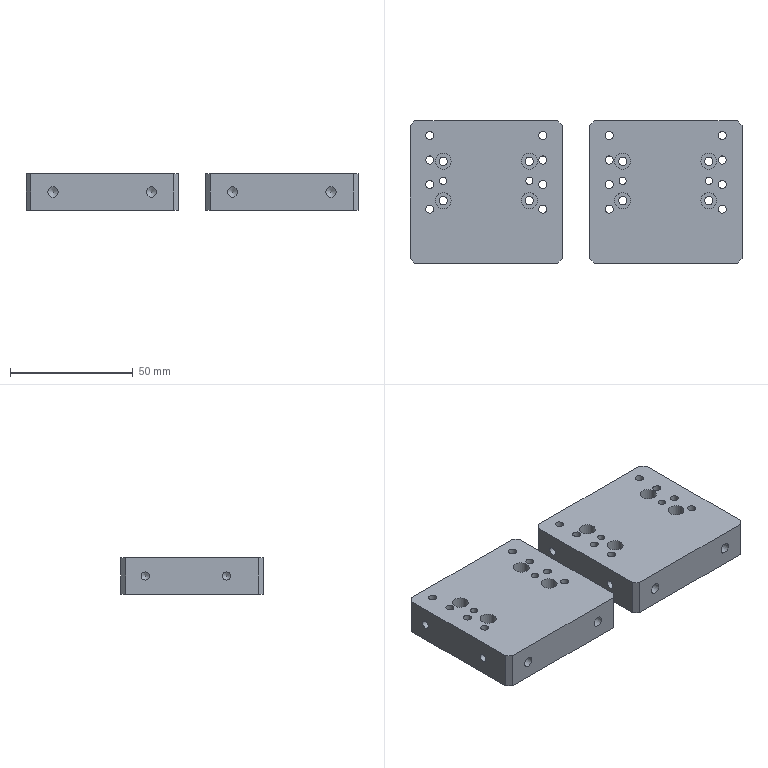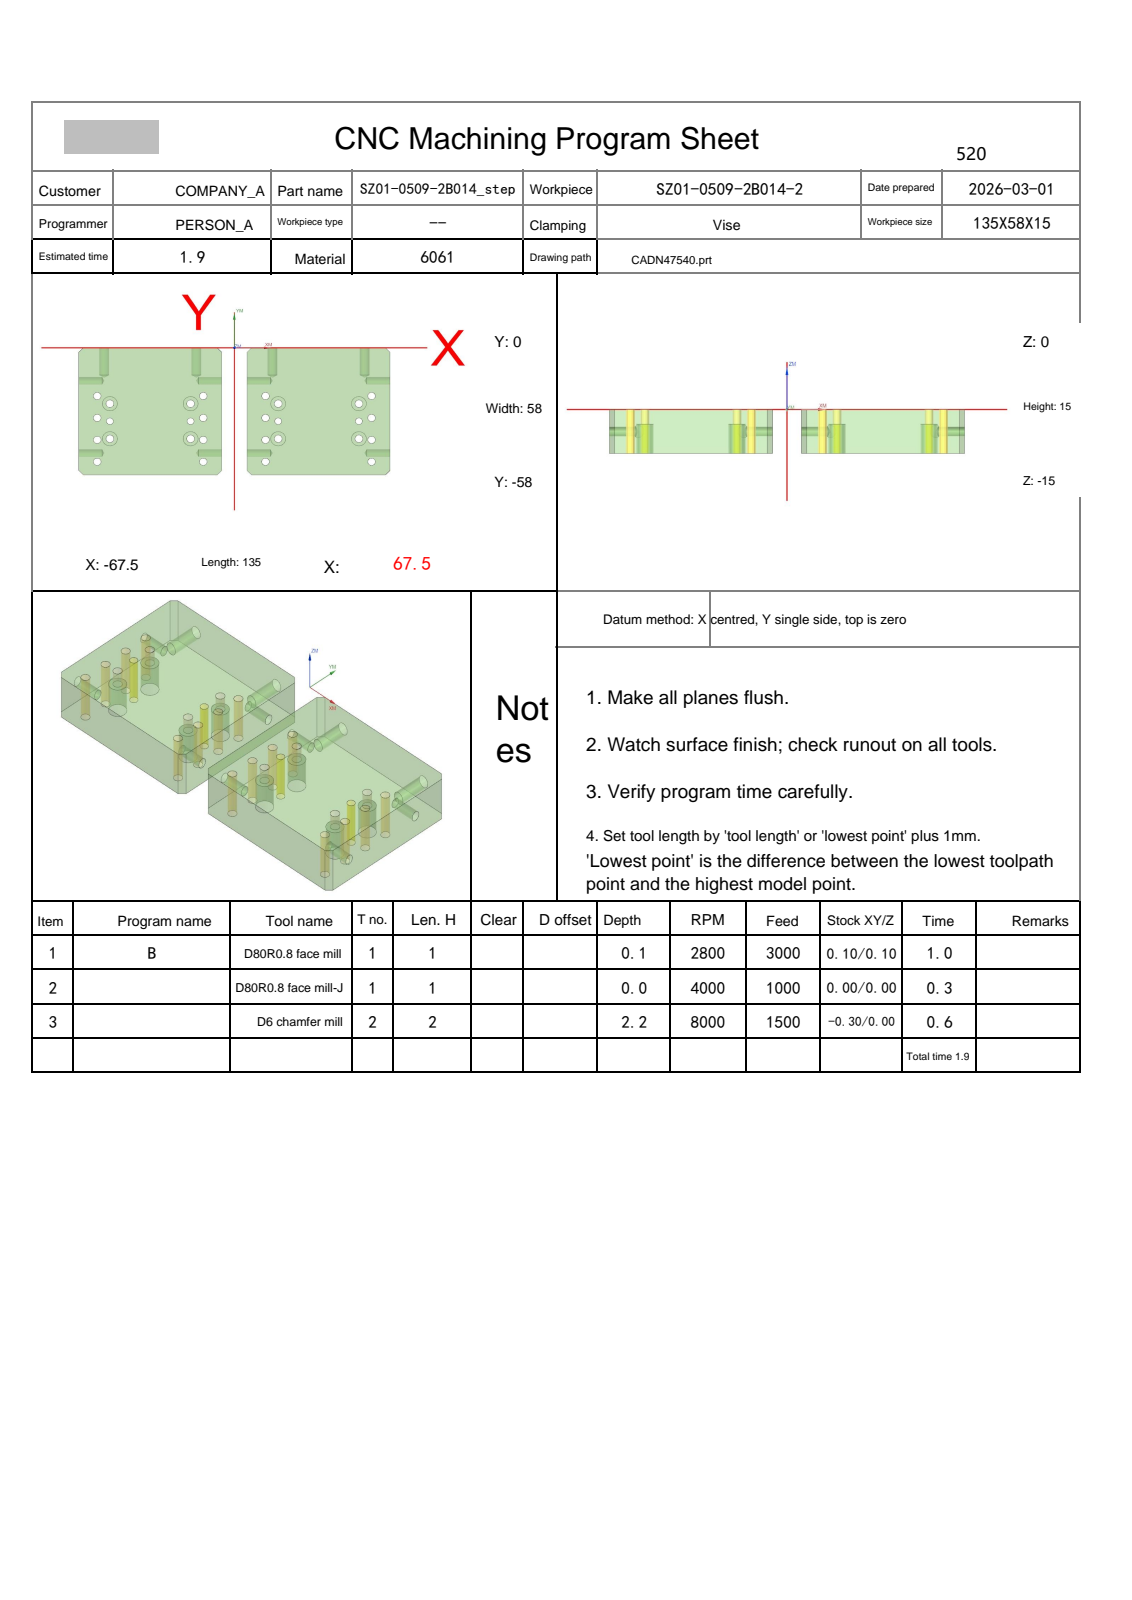NC program | NX | posted by the shop | part box 135 x 58 x 15 mm
Whole program:
%
O0001
(Machine time: 2.35 MIN)
(===Total Tool:2===)
(T1=D80R0.8 face mill D=80.  R=0.8  D-  H01 Z=0.    )
(T2=D6 chamfer mill   D=6.   R=0.   D-  H02 Z=-2.2  )
G80 G90 G17 G49 G40
G91 G28 Z0
M01
N1 T01 M06
(D80R0.8 face mill  D=80. R=0.8 H=01 ce=0.10 di=0.10)
G00 G90 G54 X119.597 Y-29. M03 S2800
G43 H01 Z50.
M08
Z6.011
G01 Z4.011 F3000.
X107.597
X-107.597
X-119.597
Z6.011
G00 X119.597
Z5.522
G01 Z3.522
X107.597
X-107.597
X-119.597
Z5.522
G00 X119.597
Z5.033
G01 Z3.033
X107.597
X-107.597
X-119.597
Z5.033
G00 X119.597
Z4.544
G01 Z2.544
X107.597
X-107.597
X-119.597
Z4.544
G00 Z50.
X119.597
Z4.056
G01 Z2.056
X107.597
X-107.597
X-119.597
Z4.056
G00 Z50.
X119.597
Z3.567
G01 Z1.567
X107.597
X-107.597
X-119.597
Z3.567
G00 Z50.
X119.597
Z3.078
G01 Z1.078
X107.597
X-107.597
X-119.597
Z3.078
G00 Z50.
X119.597
Z2.589
G01 Z.589
X107.597
X-107.597
X-119.597
Z2.589
G00 Z50.
X119.597
Z2.1
G01 Z.1
X107.597
X-107.597
X-119.597
Z2.1
G00 Z50.
G91 G28 Z0.0
M05
M09
G91 G28 Z0.0
M01
N2 T01 M06
(D80R0.8 face mill-J  D=80. R=0.8 H=01 ce=0.00 di=0.00)
G00 G90 G54 X119.499 Y-29. M03 S4000
G43 H01 Z50.
M08
Z2.
G01 Z0.0 F1000.
X107.499
X-107.499
X-119.499
Z2.
G00 Z50.
G91 G28 Z0.0
M05
M09
G91 G28 Z0.0
M01
N3 T02 M06
(D6 chamfer mill  D=6. R=0. H=02 ce=0.00 di=0.00)
G00 G90 G54 X-54. Y-33.5 M03 S8000
G43 H02 Z50.
M08
G98 G81 X-54. Y-33.5 Z-1.8 R3. F1000.
X-19.
X19.
X54.
G80
G00 Z50.
G00 G90 X-54. Y-25.5 M03 S8000
Z50.
G98 G81 X-54. Y-25.5 Z-2. R3. F1000.
Y-41.5
X-19.
Y-25.5
X19.
Y-41.5
X54.
Y-25.5
G80
G00 Z50.
G00 G90 X-59.5 Y-52. M03 S8000
Z50.
G98 G81 X-59.5 Y-52. Z-2.2 R3. F1000.
Y-42.
Y-32.
Y-22.
X-13.5
Y-32.
Y-42.
Y-52.
X13.5
Y-42.
Y-32.
Y-22.
X59.5
Y-32.
Y-42.
Y-52.
G80
G00 Z50.
G00 G90 X-68.2 Y-10.954 M03 S7000
Z50.
Z2.5
G01 Y-2.047 Z-.742 F1500.
X-68.162 Y-1.84 Z-.819
X-68.081 Y-1.645 Z-.895
X-67.962 Y-1.472 Z-.972
X-67.907 Y-1.417 Z-1.
X-66.083 Y.407
G02 X-65.376 Y.7 I.707 J-.707
G01 X-7.624
G02 X-6.917 Y.407 I0.0 J-1.
G01 X-5.093 Y-1.417
G02 X-4.8 Y-2.124 I-.707 J-.707
G01 Y-55.876
G02 X-5.093 Y-56.583 I-1. J0.0
G01 X-6.917 Y-58.407
G02 X-7.624 Y-58.7 I-.707 J.707
G01 X-65.376
G02 X-66.083 Y-58.407 I0.0 J1.
G01 X-67.907 Y-56.583
G02 X-68.2 Y-55.876 I.707 J.707
G01 Y-2.124
G02 X-67.907 Y-1.417 I1. J0.0
G01 X-67.554 Y-1.064
Z1.5
G00 Z50.
G00 G90 X4.8 Y-10.954 M03 S7000
Z50.
Z2.5
G01 Y-2.047 Z-.742 F1500.
X4.838 Y-1.84 Z-.819
X4.919 Y-1.645 Z-.895
X5.038 Y-1.472 Z-.972
X5.093 Y-1.417 Z-1.
X6.917 Y.407
G02 X7.624 Y.7 I.707 J-.707
G01 X65.376
G02 X66.083 Y.407 I0.0 J-1.
G01 X67.907 Y-1.417
G02 X68.2 Y-2.124 I-.707 J-.707
G01 Y-55.876
G02 X67.907 Y-56.583 I-1. J0.0
G01 X66.083 Y-58.407
G02 X65.376 Y-58.7 I-.707 J.707
G01 X7.624
G02 X6.917 Y-58.407 I0.0 J1.
G01 X5.093 Y-56.583
G02 X4.8 Y-55.876 I.707 J.707
G01 Y-2.124
G02 X5.093 Y-1.417 I1. J0.0
G01 X5.446 Y-1.064
Z1.5
G00 Z50.
M05
M09
G91 G28 Z0.0
G91 G28 Y0.0
M30
%